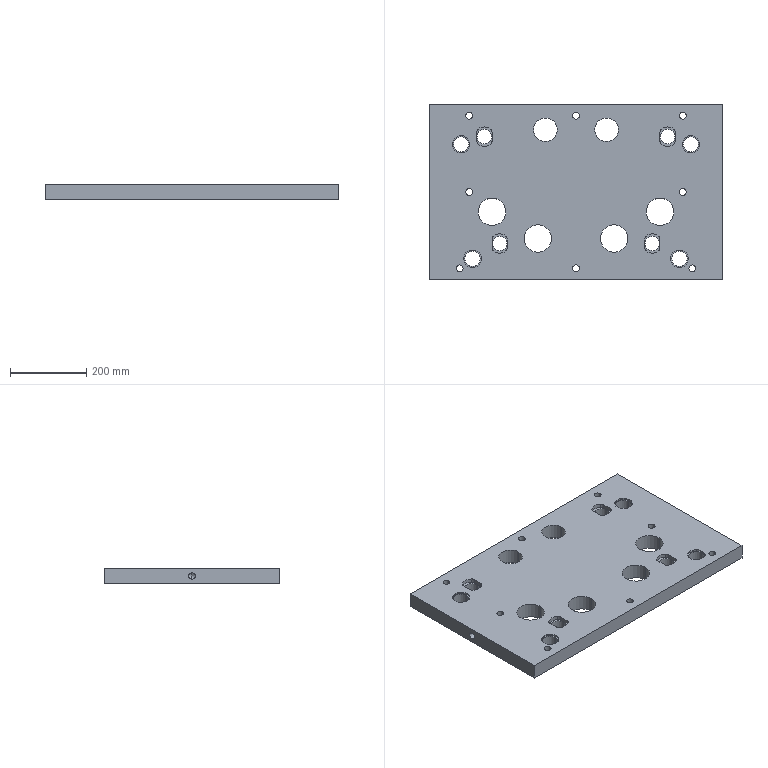Part | SolidWorks | features BaseBody 1 | 1 solid | 144 faces | box 770 x 460 x 40 mm | volume 12722716 mm3 | cylinder 96 | plane 44 | cone 4 | commonest cylinder face diameters 18 x16 20 x16 26 x16 38 x8 40 x8 46 x8